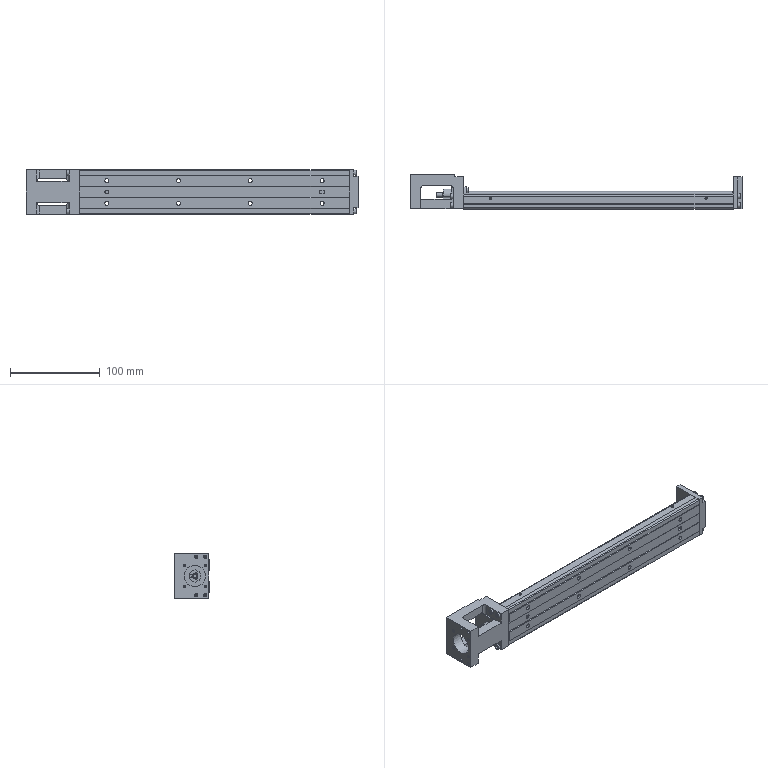Part | STEP file | C-KSC5010-B1-300-F1_b | 1 solid | 401 faces | box 370 x 38.5 x 50 mm | volume 223115 mm3 | plane 266 | cylinder 79 | cone 56 | commonest cylinder face diameters 5.5 x12 2.459 x10 4 x9 6 x9 8 x9 4.5 x8